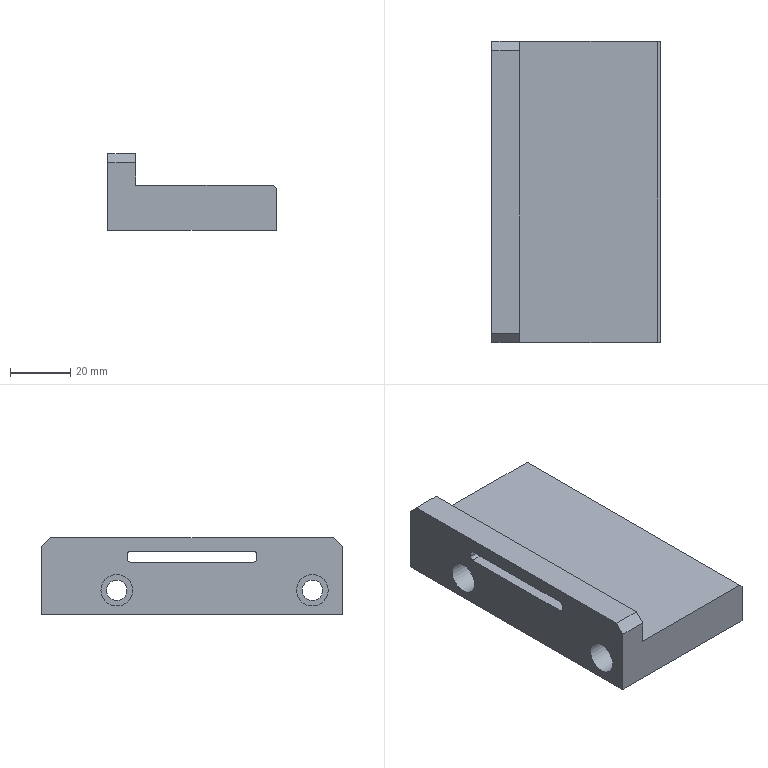Part | STEP file | Tube feed_id26_x_t | 1 solid | 25 faces | box 56 x 100 x 25.5 mm | volume 86161 mm3 | plane 17 | cylinder 8 | commonest cylinder face diameters 2 x4 6.8 x2 10.5 x2